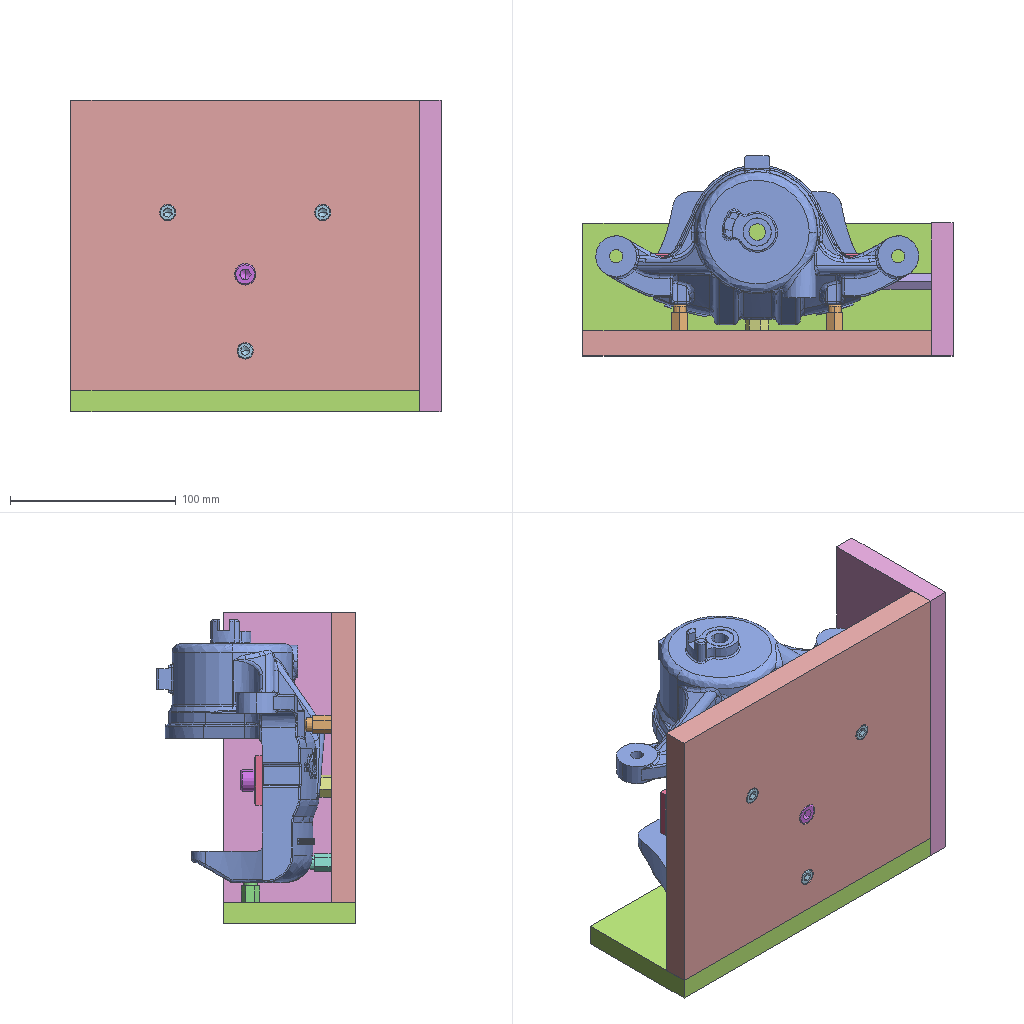Assembly | SolidWorks | 11 different items | 13 placed | box 223 x 121 x 188 mm
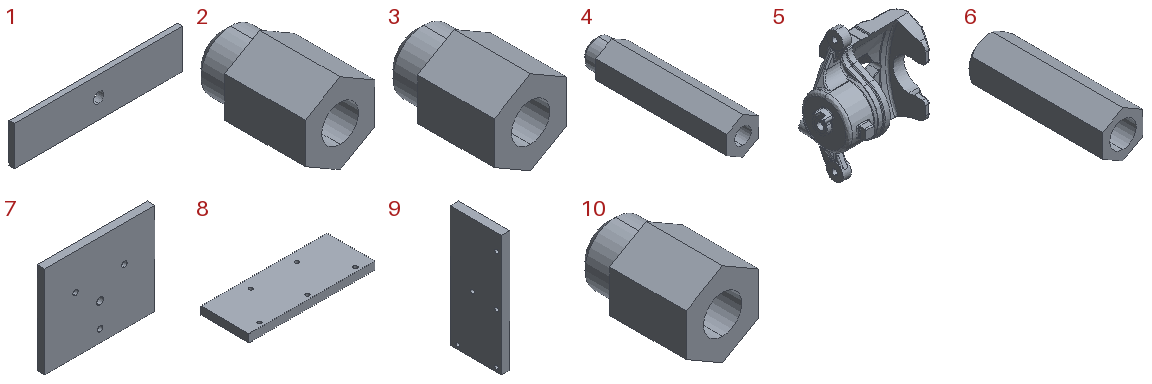Parts list (item | name | quantity | size | volume | features):
1 | - | x1 | 129 x 5 x 30 mm | 18941 mm3 | features Chamfer 1, Cut 1, Extrusion 1
2 | - | x2 | 9.526 x 16 x 11 mm | 937.407 mm3 | features Chamfer 1, Extrusion 1, HoleWzd 1, ICE 1
3 | - | x2 | 9.526 x 15 x 11 mm | 858.815 mm3 | features 3DProfileFeature 1, Chamfer 1, Extrusion 1, HoleWzd 1, ICE 1
4 | - | x1 | 9.526 x 44 x 11 mm | 3138 mm3 | features 3DProfileFeature 1, Chamfer 1, Extrusion 1, HoleWzd 1, ICE 1
5 | - | x1 | 158.2 x 101.79 x 194.7 mm | 429554 mm3 | features BaseBody 1
6 | - | x1 | 12.124 x 40.5 x 14 mm | 4147 mm3 | features ICE 3, Extrusion 1
7 | - | x1 | 210 x 15 x 175 mm | 546137 mm3 | features Cut 4, 3DProfileFeature 2, HoleWzd 2, Extrusion 1
8 | - | x1 | 210 x 80 x 13 mm | 214445 mm3 | features Cut 4, 3DProfileFeature 2, HoleWzd 2, Extrusion 1
9 | - | x1 | 13 x 80 x 188 mm | 192174 mm3 | features Cut 6, Extrusion 1
10 | - | x1 | 9.526 x 15 x 11 mm | 858.815 mm3 | features Chamfer 1, Extrusion 1, HoleWzd 1, ICE 1
11 | Socket Head Cap Screw_AM | x1 | - | - | -
Mates (type | each side: item.copy, entity, surface, feature):
Coincident | 7.1 plane | assembly plane | 3 times
Parallel | 7.1 face plane Boss-Extrude1 | 5.1 face plane Imported1 | 3 times
DistanceDim | 5.1 face plane Imported1 | 7.1 face plane Boss-Extrude1
Coincident | 7.1 face plane Boss-Extrude1 | 8.1 face plane Boss-Extrude1 | 3 times
Coincident | 7.1 face plane Boss-Extrude1 | 9.1 face plane Boss-Extrude1 | 2 times
Coincident | 8.1 face plane Boss-Extrude1 | 9.1 face plane Boss-Extrude1
DistanceDim | 5.1 face plane Imported1 | 8.1 face plane Boss-Extrude1
DistanceDim | 5.1 face plane Imported1 | 9.1 face plane Boss-Extrude1
Concentric | 7.1 face cylinder Cut-Extrude2 | 10.1 face cylinder M6x1.0 Tapped Hole1
Coincident | 7.1 face plane Boss-Extrude1 | 10.1 face plane Boss-Extrude1
Concentric | 7.1 face cylinder Cut-Extrude2 | 2.1 face cylinder M6x1.0 Tapped Hole1
Coincident | 7.1 face plane Boss-Extrude1 | 2.1 face plane Boss-Extrude1
Concentric | 7.1 face cylinder Cut-Extrude2 | 2.2 face cylinder M6x1.0 Tapped Hole1
Coincident | 7.1 face plane Boss-Extrude1 | 2.2 face plane Boss-Extrude1
Concentric | 9.1 face cylinder Cut-Extrude2 | 4.1 face cylinder M6x1.0 Tapped Hole2
Coincident | 9.1 face plane Boss-Extrude1 | 4.1 face plane Boss-Extrude1
Concentric | 8.1 face cylinder Cut-Extrude2 | 3.1 face cylinder M6x1.0 Tapped Hole2
Coincident | 8.1 face plane Boss-Extrude1 | 3.1 face plane Boss-Extrude1
Concentric | 8.1 face cylinder Cut-Extrude2 | 3.2 face cylinder M6x1.0 Tapped Hole2
Coincident | 8.1 face plane Boss-Extrude1 | 3.2 face plane Boss-Extrude1
Width | 1.1 face plane Boss-Extrude1 | 1.1 face plane Boss-Extrude1 | 5.1 face plane Imported1 | 5.1 face plane Imported1
DistanceDim | 5.1 edge | 1.1 face plane Boss-Extrude1
Concentric | 7.1 face cylinder Cut-Extrude4 | 6.1 face cylinder Cut-Extrude3
Coincident | 7.1 face plane Boss-Extrude1 | 6.1 face plane Boss-Extrude1